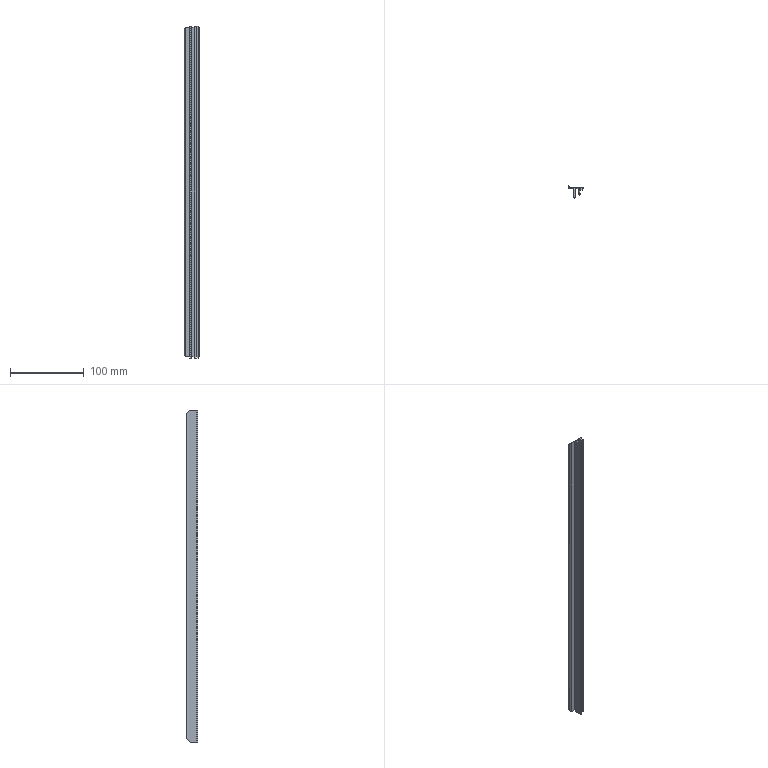Part | NX | features BREP 1 | 1 solid | 43 faces | box 21.266 x 16.173 x 450 mm | volume 30519 mm3 | plane 28 | cylinder 15 | commonest cylinder face diameters 0.585 x7 0.4 x2 1.951 x2 1.561 x1 8.16 x1 10.664 x1
STEP:
#1=CARTESIAN_POINT('',(0.,2.699,219.801));
#2=VERTEX_POINT('',#1);
#3=CARTESIAN_POINT('',(2.095,-0.55,223.05));
#4=VERTEX_POINT('',#3);
#5=CARTESIAN_POINT('',(0.,2.699,219.801));
#6=CARTESIAN_POINT('',(0.2706,1.376,221.124));
#7=CARTESIAN_POINT('',(1.002,0.242,222.258));
#8=CARTESIAN_POINT('',(2.095,-0.55,223.05));
#9=(BOUNDED_CURVE()B_SPLINE_CURVE(3,(#5,#6,#7,#8),.UNSPECIFIED.,.F.,.F.)B_SPLINE_CURVE_WITH_KNOTS((4,4),(1.773,2.515),.UNSPECIFIED.)CURVE()GEOMETRIC_REPRESENTATION_ITEM()RATIONAL_B_SPLINE_CURVE((1.,0.9547,0.9547,1.))REPRESENTATION_ITEM(''));
#10=EDGE_CURVE('',#2,#4,#9,.T.);
#11=ORIENTED_EDGE('',*,*,#10,.F.);
#12=CARTESIAN_POINT('',(0.,2.699,-219.801));
#13=VERTEX_POINT('',#12);
#14=CARTESIAN_POINT('',(0.,2.699,225.));
#15=DIRECTION('',(0.,0.,-1.));
#16=VECTOR('',#15,1000.);
#17=LINE('',#14,#16);
#18=EDGE_CURVE('',#2,#13,#17,.T.);
#19=ORIENTED_EDGE('',*,*,#18,.T.);
#20=CARTESIAN_POINT('',(2.095,-0.55,-223.05));
#21=VERTEX_POINT('',#20);
#22=CARTESIAN_POINT('',(2.095,-0.55,-223.05));
#23=CARTESIAN_POINT('',(1.002,0.242,-222.258));
#24=CARTESIAN_POINT('',(0.2706,1.376,-221.124));
#25=CARTESIAN_POINT('',(0.,2.699,-219.801));
#26=(BOUNDED_CURVE()B_SPLINE_CURVE(3,(#22,#23,#24,#25),.UNSPECIFIED.,.F.,.F.)B_SPLINE_CURVE_WITH_KNOTS((4,4),(0.6271,1.369),.UNSPECIFIED.)CURVE()GEOMETRIC_REPRESENTATION_ITEM()RATIONAL_B_SPLINE_CURVE((1.,0.9547,0.9547,1.))REPRESENTATION_ITEM(''));
#27=EDGE_CURVE('',#21,#13,#26,.T.);
#28=ORIENTED_EDGE('',*,*,#27,.F.);
#29=CARTESIAN_POINT('',(2.095,-0.55,225.));
#30=DIRECTION('',(0.,0.,-1.));
#31=VECTOR('',#30,1000.);
#32=LINE('',#29,#31);
#33=EDGE_CURVE('',#4,#21,#32,.T.);
#34=ORIENTED_EDGE('',*,*,#33,.F.);
#35=EDGE_LOOP('',(#11,#19,#28,#34));
#36=FACE_BOUND('',#35,.T.);
#37=CARTESIAN_POINT('',(5.224,3.768,225.));
#38=DIRECTION('',(0.,0.,-1.));
#39=DIRECTION('',(-1.,0.,0.));
#40=AXIS2_PLACEMENT_3D('',#37,#38,#39);
#41=CYLINDRICAL_SURFACE('',#40,5.332);
#42=ADVANCED_FACE('',(#36),#41,.T.);
#43=CARTESIAN_POINT('',(7.9,-0.55,223.05));
#44=VERTEX_POINT('',#43);
#45=CARTESIAN_POINT('',(2.095,-0.55,223.05));
#46=DIRECTION('',(1.,0.,0.));
#47=VECTOR('',#46,1000.);
#48=LINE('',#45,#47);
#49=EDGE_CURVE('',#4,#44,#48,.T.);
#50=ORIENTED_EDGE('',*,*,#49,.F.);
#51=ORIENTED_EDGE('',*,*,#33,.T.);
#52=CARTESIAN_POINT('',(7.9,-0.55,-223.05));
#53=VERTEX_POINT('',#52);
#54=CARTESIAN_POINT('',(2.095,-0.55,-223.05));
#55=DIRECTION('',(-1.,0.,0.));
#56=VECTOR('',#55,1000.);
#57=LINE('',#54,#56);
#58=EDGE_CURVE('',#53,#21,#57,.T.);
#59=ORIENTED_EDGE('',*,*,#58,.F.);
#60=CARTESIAN_POINT('',(7.9,-0.55,225.));
#61=DIRECTION('',(0.,0.,-1.));
#62=VECTOR('',#61,1000.);
#63=LINE('',#60,#62);
#64=EDGE_CURVE('',#44,#53,#63,.T.);
#65=ORIENTED_EDGE('',*,*,#64,.F.);
#66=EDGE_LOOP('',(#50,#51,#59,#65));
#67=FACE_BOUND('',#66,.T.);
#68=CARTESIAN_POINT('',(2.095,-0.55,225.));
#69=DIRECTION('',(0.,1.,0.));
#70=DIRECTION('',(1.,0.,0.));
#71=AXIS2_PLACEMENT_3D('',#68,#69,#70);
#72=PLANE('',#71);
#73=ADVANCED_FACE('',(#67),#72,.F.);
#74=CARTESIAN_POINT('',(7.9,-2.5,225.));
#75=VERTEX_POINT('',#74);
#76=CARTESIAN_POINT('',(7.9,-1.525,224.025));
#77=DIRECTION('',(0.,-0.7071,0.7071));
#78=VECTOR('',#77,1000.);
#79=LINE('',#76,#78);
#80=EDGE_CURVE('',#44,#75,#79,.T.);
#81=ORIENTED_EDGE('',*,*,#80,.F.);
#82=ORIENTED_EDGE('',*,*,#64,.T.);
#83=CARTESIAN_POINT('',(7.9,-2.5,-225.));
#84=VERTEX_POINT('',#83);
#85=CARTESIAN_POINT('',(7.9,223.475,0.975));
#86=DIRECTION('',(0.,0.7071,0.7071));
#87=VECTOR('',#86,1000.);
#88=LINE('',#85,#87);
#89=EDGE_CURVE('',#84,#53,#88,.T.);
#90=ORIENTED_EDGE('',*,*,#89,.F.);
#91=CARTESIAN_POINT('',(7.9,-11.847,-225.));
#92=VERTEX_POINT('',#91);
#93=CARTESIAN_POINT('',(7.9,-0.55,-225.));
#94=DIRECTION('',(0.,-1.,0.));
#95=VECTOR('',#94,1000.);
#96=LINE('',#93,#95);
#97=EDGE_CURVE('',#84,#92,#96,.T.);
#98=ORIENTED_EDGE('',*,*,#97,.T.);
#99=CARTESIAN_POINT('',(7.9,-11.847,225.));
#100=VERTEX_POINT('',#99);
#101=CARTESIAN_POINT('',(7.9,-11.847,225.));
#102=DIRECTION('',(0.,0.,-1.));
#103=VECTOR('',#102,1000.);
#104=LINE('',#101,#103);
#105=EDGE_CURVE('',#100,#92,#104,.T.);
#106=ORIENTED_EDGE('',*,*,#105,.F.);
#107=CARTESIAN_POINT('',(7.9,-0.55,225.));
#108=DIRECTION('',(0.,-1.,0.));
#109=VECTOR('',#108,1000.);
#110=LINE('',#107,#109);
#111=EDGE_CURVE('',#75,#100,#110,.T.);
#112=ORIENTED_EDGE('',*,*,#111,.F.);
#113=EDGE_LOOP('',(#81,#82,#90,#98,#106,#112));
#114=FACE_BOUND('',#113,.T.);
#115=CARTESIAN_POINT('',(7.9,-0.55,225.));
#116=DIRECTION('',(1.,0.,0.));
#117=DIRECTION('',(0.,1.,0.));
#118=AXIS2_PLACEMENT_3D('',#115,#116,#117);
#119=PLANE('',#118);
#120=ADVANCED_FACE('',(#114),#119,.F.);
#121=CARTESIAN_POINT('',(9.363,-2.5,225.));
#122=VERTEX_POINT('',#121);
#123=CARTESIAN_POINT('',(9.363,-1.526,224.026));
#124=VERTEX_POINT('',#123);
#125=CARTESIAN_POINT('',(9.363,-7.399,229.899));
#126=DIRECTION('',(0.,0.7071,-0.7071));
#127=VECTOR('',#126,1000.);
#128=LINE('',#125,#127);
#129=EDGE_CURVE('',#122,#124,#128,.T.);
#130=ORIENTED_EDGE('',*,*,#129,.F.);
#131=CARTESIAN_POINT('',(9.363,-12.298,225.));
#132=VERTEX_POINT('',#131);
#133=CARTESIAN_POINT('',(9.363,-12.298,225.));
#134=DIRECTION('',(0.,1.,0.));
#135=VECTOR('',#134,1000.);
#136=LINE('',#133,#135);
#137=EDGE_CURVE('',#132,#122,#136,.T.);
#138=ORIENTED_EDGE('',*,*,#137,.F.);
#139=CARTESIAN_POINT('',(9.363,-12.298,-225.));
#140=VERTEX_POINT('',#139);
#141=CARTESIAN_POINT('',(9.363,-12.298,225.));
#142=DIRECTION('',(0.,0.,-1.));
#143=VECTOR('',#142,1000.);
#144=LINE('',#141,#143);
#145=EDGE_CURVE('',#132,#140,#144,.T.);
#146=ORIENTED_EDGE('',*,*,#145,.T.);
#147=CARTESIAN_POINT('',(9.363,-2.5,-225.));
#148=VERTEX_POINT('',#147);
#149=CARTESIAN_POINT('',(9.363,-12.298,-225.));
#150=DIRECTION('',(0.,1.,0.));
#151=VECTOR('',#150,1000.);
#152=LINE('',#149,#151);
#153=EDGE_CURVE('',#140,#148,#152,.T.);
#154=ORIENTED_EDGE('',*,*,#153,.T.);
#155=CARTESIAN_POINT('',(9.363,-1.526,-224.026));
#156=VERTEX_POINT('',#155);
#157=CARTESIAN_POINT('',(9.363,217.601,-4.899));
#158=DIRECTION('',(0.,-0.7071,-0.7071));
#159=VECTOR('',#158,1000.);
#160=LINE('',#157,#159);
#161=EDGE_CURVE('',#156,#148,#160,.T.);
#162=ORIENTED_EDGE('',*,*,#161,.F.);
#163=CARTESIAN_POINT('',(9.363,-1.526,225.));
#164=DIRECTION('',(0.,0.,-1.));
#165=VECTOR('',#164,1000.);
#166=LINE('',#163,#165);
#167=EDGE_CURVE('',#124,#156,#166,.T.);
#168=ORIENTED_EDGE('',*,*,#167,.F.);
#169=EDGE_LOOP('',(#130,#138,#146,#154,#162,#168));
#170=FACE_BOUND('',#169,.T.);
#171=CARTESIAN_POINT('',(9.363,-12.298,225.));
#172=DIRECTION('',(-1.,0.,0.));
#173=DIRECTION('',(0.,0.,1.));
#174=AXIS2_PLACEMENT_3D('',#171,#172,#173);
#175=PLANE('',#174);
#176=ADVANCED_FACE('',(#170),#175,.F.);
#177=CARTESIAN_POINT('',(10.339,-0.55,223.05));
#178=VERTEX_POINT('',#177);
#179=CARTESIAN_POINT('',(9.363,-1.526,224.026));
#180=CARTESIAN_POINT('',(9.363,-0.9541,223.454));
#181=CARTESIAN_POINT('',(9.768,-0.55,223.05));
#182=CARTESIAN_POINT('',(10.339,-0.55,223.05));
#183=(BOUNDED_CURVE()B_SPLINE_CURVE(3,(#179,#180,#181,#182),.UNSPECIFIED.,.F.,.F.)B_SPLINE_CURVE_WITH_KNOTS((4,4),(4.712,6.283),.UNSPECIFIED.)CURVE()GEOMETRIC_REPRESENTATION_ITEM()RATIONAL_B_SPLINE_CURVE((1.,0.8047,0.8047,1.))REPRESENTATION_ITEM(''));
#184=EDGE_CURVE('',#124,#178,#183,.T.);
#185=ORIENTED_EDGE('',*,*,#184,.F.);
#186=ORIENTED_EDGE('',*,*,#167,.T.);
#187=CARTESIAN_POINT('',(10.339,-0.55,-223.05));
#188=VERTEX_POINT('',#187);
#189=CARTESIAN_POINT('',(10.339,-0.55,-223.05));
#190=CARTESIAN_POINT('',(9.768,-0.55,-223.05));
#191=CARTESIAN_POINT('',(9.363,-0.9541,-223.454));
#192=CARTESIAN_POINT('',(9.363,-1.526,-224.026));
#193=(BOUNDED_CURVE()B_SPLINE_CURVE(3,(#189,#190,#191,#192),.UNSPECIFIED.,.F.,.F.)B_SPLINE_CURVE_WITH_KNOTS((4,4),(3.142,4.712),.UNSPECIFIED.)CURVE()GEOMETRIC_REPRESENTATION_ITEM()RATIONAL_B_SPLINE_CURVE((1.,0.8047,0.8047,1.))REPRESENTATION_ITEM(''));
#194=EDGE_CURVE('',#188,#156,#193,.T.);
#195=ORIENTED_EDGE('',*,*,#194,.F.);
#196=CARTESIAN_POINT('',(10.339,-0.55,225.));
#197=DIRECTION('',(0.,0.,-1.));
#198=VECTOR('',#197,1000.);
#199=LINE('',#196,#198);
#200=EDGE_CURVE('',#178,#188,#199,.T.);
#201=ORIENTED_EDGE('',*,*,#200,.F.);
#202=EDGE_LOOP('',(#185,#186,#195,#201));
#203=FACE_BOUND('',#202,.T.);
#204=CARTESIAN_POINT('',(10.339,-1.526,225.));
#205=DIRECTION('',(0.,0.,-1.));
#206=DIRECTION('',(-1.,0.,0.));
#207=AXIS2_PLACEMENT_3D('',#204,#205,#206);
#208=CYLINDRICAL_SURFACE('',#207,0.9756);
#209=ADVANCED_FACE('',(#203),#208,.F.);
#210=CARTESIAN_POINT('',(13.461,-0.55,223.05));
#211=VERTEX_POINT('',#210);
#212=CARTESIAN_POINT('',(10.339,-0.55,223.05));
#213=DIRECTION('',(1.,0.,0.));
#214=VECTOR('',#213,1000.);
#215=LINE('',#212,#214);
#216=EDGE_CURVE('',#178,#211,#215,.T.);
#217=ORIENTED_EDGE('',*,*,#216,.F.);
#218=ORIENTED_EDGE('',*,*,#200,.T.);
#219=CARTESIAN_POINT('',(13.461,-0.55,-223.05));
#220=VERTEX_POINT('',#219);
#221=CARTESIAN_POINT('',(10.339,-0.55,-223.05));
#222=DIRECTION('',(-1.,0.,0.));
#223=VECTOR('',#222,1000.);
#224=LINE('',#221,#223);
#225=EDGE_CURVE('',#220,#188,#224,.T.);
#226=ORIENTED_EDGE('',*,*,#225,.F.);
#227=CARTESIAN_POINT('',(13.461,-0.55,225.));
#228=DIRECTION('',(0.,0.,-1.));
#229=VECTOR('',#228,1000.);
#230=LINE('',#227,#229);
#231=EDGE_CURVE('',#211,#220,#230,.T.);
#232=ORIENTED_EDGE('',*,*,#231,.F.);
#233=EDGE_LOOP('',(#217,#218,#226,#232));
#234=FACE_BOUND('',#233,.T.);
#235=CARTESIAN_POINT('',(10.339,-0.55,225.));
#236=DIRECTION('',(0.,1.,0.));
#237=DIRECTION('',(1.,0.,0.));
#238=AXIS2_PLACEMENT_3D('',#235,#236,#237);
#239=PLANE('',#238);
#240=ADVANCED_FACE('',(#234),#239,.F.);
#241=CARTESIAN_POINT('',(14.437,-1.526,224.026));
#242=VERTEX_POINT('',#241);
#243=CARTESIAN_POINT('',(13.461,-0.55,223.05));
#244=CARTESIAN_POINT('',(14.032,-0.55,223.05));
#245=CARTESIAN_POINT('',(14.437,-0.9541,223.454));
#246=CARTESIAN_POINT('',(14.437,-1.526,224.026));
#247=(BOUNDED_CURVE()B_SPLINE_CURVE(3,(#243,#244,#245,#246),.UNSPECIFIED.,.F.,.F.)B_SPLINE_CURVE_WITH_KNOTS((4,4),(0.,1.571),.UNSPECIFIED.)CURVE()GEOMETRIC_REPRESENTATION_ITEM()RATIONAL_B_SPLINE_CURVE((1.,0.8047,0.8047,1.))REPRESENTATION_ITEM(''));
#248=EDGE_CURVE('',#211,#242,#247,.T.);
#249=ORIENTED_EDGE('',*,*,#248,.F.);
#250=ORIENTED_EDGE('',*,*,#231,.T.);
#251=CARTESIAN_POINT('',(14.437,-1.526,-224.026));
#252=VERTEX_POINT('',#251);
#253=CARTESIAN_POINT('',(14.437,-1.526,-224.026));
#254=CARTESIAN_POINT('',(14.437,-0.9541,-223.454));
#255=CARTESIAN_POINT('',(14.032,-0.55,-223.05));
#256=CARTESIAN_POINT('',(13.461,-0.55,-223.05));
#257=(BOUNDED_CURVE()B_SPLINE_CURVE(3,(#253,#254,#255,#256),.UNSPECIFIED.,.F.,.F.)B_SPLINE_CURVE_WITH_KNOTS((4,4),(1.571,3.142),.UNSPECIFIED.)CURVE()GEOMETRIC_REPRESENTATION_ITEM()RATIONAL_B_SPLINE_CURVE((1.,0.8047,0.8047,1.))REPRESENTATION_ITEM(''));
#258=EDGE_CURVE('',#252,#220,#257,.T.);
#259=ORIENTED_EDGE('',*,*,#258,.F.);
#260=CARTESIAN_POINT('',(14.437,-1.526,225.));
#261=DIRECTION('',(0.,0.,-1.));
#262=VECTOR('',#261,1000.);
#263=LINE('',#260,#262);
#264=EDGE_CURVE('',#242,#252,#263,.T.);
#265=ORIENTED_EDGE('',*,*,#264,.F.);
#266=EDGE_LOOP('',(#249,#250,#259,#265));
#267=FACE_BOUND('',#266,.T.);
#268=CARTESIAN_POINT('',(13.461,-1.526,225.));
#269=DIRECTION('',(0.,0.,-1.));
#270=DIRECTION('',(-1.,0.,0.));
#271=AXIS2_PLACEMENT_3D('',#268,#269,#270);
#272=CYLINDRICAL_SURFACE('',#271,0.9756);
#273=ADVANCED_FACE('',(#267),#272,.F.);
#274=CARTESIAN_POINT('',(14.437,-2.5,225.));
#275=VERTEX_POINT('',#274);
#276=CARTESIAN_POINT('',(14.437,-2.013,224.513));
#277=DIRECTION('',(0.,-0.7071,0.7071));
#278=VECTOR('',#277,1000.);
#279=LINE('',#276,#278);
#280=EDGE_CURVE('',#242,#275,#279,.T.);
#281=ORIENTED_EDGE('',*,*,#280,.F.);
#282=ORIENTED_EDGE('',*,*,#264,.T.);
#283=CARTESIAN_POINT('',(14.437,-2.5,-225.));
#284=VERTEX_POINT('',#283);
#285=CARTESIAN_POINT('',(14.437,222.987,0.4872));
#286=DIRECTION('',(0.,0.7071,0.7071));
#287=VECTOR('',#286,1000.);
#288=LINE('',#285,#287);
#289=EDGE_CURVE('',#284,#252,#288,.T.);
#290=ORIENTED_EDGE('',*,*,#289,.F.);
#291=CARTESIAN_POINT('',(14.437,-8.128,-225.));
#292=VERTEX_POINT('',#291);
#293=CARTESIAN_POINT('',(14.437,-1.526,-225.));
#294=DIRECTION('',(0.,-1.,0.));
#295=VECTOR('',#294,1000.);
#296=LINE('',#293,#295);
#297=EDGE_CURVE('',#284,#292,#296,.T.);
#298=ORIENTED_EDGE('',*,*,#297,.T.);
#299=CARTESIAN_POINT('',(14.437,-8.128,225.));
#300=VERTEX_POINT('',#299);
#301=CARTESIAN_POINT('',(14.437,-8.128,225.));
#302=DIRECTION('',(0.,0.,-1.));
#303=VECTOR('',#302,1000.);
#304=LINE('',#301,#303);
#305=EDGE_CURVE('',#300,#292,#304,.T.);
#306=ORIENTED_EDGE('',*,*,#305,.F.);
#307=CARTESIAN_POINT('',(14.437,-1.526,225.));
#308=DIRECTION('',(0.,-1.,0.));
#309=VECTOR('',#308,1000.);
#310=LINE('',#307,#309);
#311=EDGE_CURVE('',#275,#300,#310,.T.);
#312=ORIENTED_EDGE('',*,*,#311,.F.);
#313=EDGE_LOOP('',(#281,#282,#290,#298,#306,#312));
#314=FACE_BOUND('',#313,.T.);
#315=CARTESIAN_POINT('',(14.437,-1.526,225.));
#316=DIRECTION('',(1.,0.,0.));
#317=DIRECTION('',(0.,1.,0.));
#318=AXIS2_PLACEMENT_3D('',#315,#316,#317);
#319=PLANE('',#318);
#320=ADVANCED_FACE('',(#314),#319,.F.);
#321=CARTESIAN_POINT('',(15.9,-2.5,225.));
#322=VERTEX_POINT('',#321);
#323=CARTESIAN_POINT('',(15.9,-0.55,223.05));
#324=VERTEX_POINT('',#323);
#325=CARTESIAN_POINT('',(15.9,-4.93,227.43));
#326=DIRECTION('',(0.,0.7071,-0.7071));
#327=VECTOR('',#326,1000.);
#328=LINE('',#325,#327);
#329=EDGE_CURVE('',#322,#324,#328,.T.);
#330=ORIENTED_EDGE('',*,*,#329,.F.);
#331=CARTESIAN_POINT('',(15.9,-7.36,225.));
#332=VERTEX_POINT('',#331);
#333=CARTESIAN_POINT('',(15.9,-7.36,225.));
#334=DIRECTION('',(0.,1.,0.));
#335=VECTOR('',#334,1000.);
#336=LINE('',#333,#335);
#337=EDGE_CURVE('',#332,#322,#336,.T.);
#338=ORIENTED_EDGE('',*,*,#337,.F.);
#339=CARTESIAN_POINT('',(15.9,-7.36,-225.));
#340=VERTEX_POINT('',#339);
#341=CARTESIAN_POINT('',(15.9,-7.36,225.));
#342=DIRECTION('',(0.,0.,-1.));
#343=VECTOR('',#342,1000.);
#344=LINE('',#341,#343);
#345=EDGE_CURVE('',#332,#340,#344,.T.);
#346=ORIENTED_EDGE('',*,*,#345,.T.);
#347=CARTESIAN_POINT('',(15.9,-2.5,-225.));
#348=VERTEX_POINT('',#347);
#349=CARTESIAN_POINT('',(15.9,-7.36,-225.));
#350=DIRECTION('',(0.,1.,0.));
#351=VECTOR('',#350,1000.);
#352=LINE('',#349,#351);
#353=EDGE_CURVE('',#340,#348,#352,.T.);
#354=ORIENTED_EDGE('',*,*,#353,.T.);
#355=CARTESIAN_POINT('',(15.9,-0.55,-223.05));
#356=VERTEX_POINT('',#355);
#357=CARTESIAN_POINT('',(15.9,220.07,-2.43));
#358=DIRECTION('',(0.,-0.7071,-0.7071));
#359=VECTOR('',#358,1000.);
#360=LINE('',#357,#359);
#361=EDGE_CURVE('',#356,#348,#360,.T.);
#362=ORIENTED_EDGE('',*,*,#361,.F.);
#363=CARTESIAN_POINT('',(15.9,-0.55,225.));
#364=DIRECTION('',(0.,0.,-1.));
#365=VECTOR('',#364,1000.);
#366=LINE('',#363,#365);
#367=EDGE_CURVE('',#324,#356,#366,.T.);
#368=ORIENTED_EDGE('',*,*,#367,.F.);
#369=EDGE_LOOP('',(#330,#338,#346,#354,#362,#368));
#370=FACE_BOUND('',#369,.T.);
#371=CARTESIAN_POINT('',(15.9,-7.36,225.));
#372=DIRECTION('',(-1.,0.,0.));
#373=DIRECTION('',(0.,0.,1.));
#374=AXIS2_PLACEMENT_3D('',#371,#372,#373);
#375=PLANE('',#374);
#376=ADVANCED_FACE('',(#370),#375,.F.);
#377=CARTESIAN_POINT('',(17.363,-0.55,223.05));
#378=VERTEX_POINT('',#377);
#379=CARTESIAN_POINT('',(15.9,-0.55,223.05));
#380=DIRECTION('',(1.,0.,0.));
#381=VECTOR('',#380,1000.);
#382=LINE('',#379,#381);
#383=EDGE_CURVE('',#324,#378,#382,.T.);
#384=ORIENTED_EDGE('',*,*,#383,.F.);
#385=ORIENTED_EDGE('',*,*,#367,.T.);
#386=CARTESIAN_POINT('',(17.363,-0.55,-223.05));
#387=VERTEX_POINT('',#386);
#388=CARTESIAN_POINT('',(15.9,-0.55,-223.05));
#389=DIRECTION('',(-1.,0.,0.));
#390=VECTOR('',#389,1000.);
#391=LINE('',#388,#390);
#392=EDGE_CURVE('',#387,#356,#391,.T.);
#393=ORIENTED_EDGE('',*,*,#392,.F.);
#394=CARTESIAN_POINT('',(17.363,-0.55,225.));
#395=DIRECTION('',(0.,0.,-1.));
#396=VECTOR('',#395,1000.);
#397=LINE('',#394,#396);
#398=EDGE_CURVE('',#378,#387,#397,.T.);
#399=ORIENTED_EDGE('',*,*,#398,.F.);
#400=EDGE_LOOP('',(#384,#385,#393,#399));
#401=FACE_BOUND('',#400,.T.);
#402=CARTESIAN_POINT('',(15.9,-0.55,225.));
#403=DIRECTION('',(0.,1.,0.));
#404=DIRECTION('',(1.,0.,0.));
#405=AXIS2_PLACEMENT_3D('',#402,#403,#404);
#406=PLANE('',#405);
#407=ADVANCED_FACE('',(#401),#406,.F.);
#408=CARTESIAN_POINT('',(17.363,-2.5,225.));
#409=VERTEX_POINT('',#408);
#410=CARTESIAN_POINT('',(17.363,-1.525,224.025));
#411=DIRECTION('',(0.,-0.7071,0.7071));
#412=VECTOR('',#411,1000.);
#413=LINE('',#410,#412);
#414=EDGE_CURVE('',#378,#409,#413,.T.);
#415=ORIENTED_EDGE('',*,*,#414,.F.);
#416=ORIENTED_EDGE('',*,*,#398,.T.);
#417=CARTESIAN_POINT('',(17.363,-2.5,-225.));
#418=VERTEX_POINT('',#417);
#419=CARTESIAN_POINT('',(17.363,223.475,0.975));
#420=DIRECTION('',(0.,0.7071,0.7071));
#421=VECTOR('',#420,1000.);
#422=LINE('',#419,#421);
#423=EDGE_CURVE('',#418,#387,#422,.T.);
#424=ORIENTED_EDGE('',*,*,#423,.F.);
#425=CARTESIAN_POINT('',(17.363,-2.501,-225.));
#426=VERTEX_POINT('',#425);
#427=CARTESIAN_POINT('',(17.363,-0.55,-225.));
#428=DIRECTION('',(0.,-1.,0.));
#429=VECTOR('',#428,1000.);
#430=LINE('',#427,#429);
#431=EDGE_CURVE('',#418,#426,#430,.T.);
#432=ORIENTED_EDGE('',*,*,#431,.T.);
#433=CARTESIAN_POINT('',(17.363,-2.501,225.));
#434=VERTEX_POINT('',#433);
#435=CARTESIAN_POINT('',(17.363,-2.501,225.));
#436=DIRECTION('',(0.,0.,-1.));
#437=VECTOR('',#436,1000.);
#438=LINE('',#435,#437);
#439=EDGE_CURVE('',#434,#426,#438,.T.);
#440=ORIENTED_EDGE('',*,*,#439,.F.);
#441=CARTESIAN_POINT('',(17.363,-0.55,225.));
#442=DIRECTION('',(0.,-1.,0.));
#443=VECTOR('',#442,1000.);
#444=LINE('',#441,#443);
#445=EDGE_CURVE('',#409,#434,#444,.T.);
#446=ORIENTED_EDGE('',*,*,#445,.F.);
#447=EDGE_LOOP('',(#415,#416,#424,#432,#440,#446));
#448=FACE_BOUND('',#447,.T.);
#449=CARTESIAN_POINT('',(17.363,-0.55,225.));
#450=DIRECTION('',(1.,0.,0.));
#451=DIRECTION('',(0.,1.,0.));
#452=AXIS2_PLACEMENT_3D('',#449,#450,#451);
#453=PLANE('',#452);
#454=ADVANCED_FACE('',(#448),#453,.F.);
#455=CARTESIAN_POINT('',(19.049,-2.5,225.));
#456=VERTEX_POINT('',#455);
#457=CARTESIAN_POINT('',(19.315,-2.209,224.709));
#458=VERTEX_POINT('',#457);
#459=CARTESIAN_POINT('',(19.049,-2.5,225.));
#460=CARTESIAN_POINT('',(19.207,-2.485,224.985));
#461=CARTESIAN_POINT('',(19.315,-2.368,224.868));
#462=CARTESIAN_POINT('',(19.315,-2.209,224.709));
#463=(BOUNDED_CURVE()B_SPLINE_CURVE(3,(#459,#460,#461,#462),.UNSPECIFIED.,.F.,.F.)B_SPLINE_CURVE_WITH_KNOTS((4,4),(3.233,4.712),.UNSPECIFIED.)CURVE()GEOMETRIC_REPRESENTATION_ITEM()RATIONAL_B_SPLINE_CURVE((1.,0.8258,0.8258,1.))REPRESENTATION_ITEM(''));
#464=EDGE_CURVE('',#456,#458,#463,.T.);
#465=ORIENTED_EDGE('',*,*,#464,.F.);
#466=CARTESIAN_POINT('',(19.022,-2.501,225.));
#467=VERTEX_POINT('',#466);
#468=CARTESIAN_POINT('',(19.022,-2.209,225.));
#469=DIRECTION('',(0.,0.,1.));
#470=DIRECTION('',(1.,0.,0.));
#471=AXIS2_PLACEMENT_3D('',#468,#469,#470);
#472=CIRCLE('',#471,0.2927);
#473=EDGE_CURVE('',#467,#456,#472,.T.);
#474=ORIENTED_EDGE('',*,*,#473,.F.);
#475=CARTESIAN_POINT('',(19.022,-2.501,-225.));
#476=VERTEX_POINT('',#475);
#477=CARTESIAN_POINT('',(19.022,-2.501,225.));
#478=DIRECTION('',(0.,0.,-1.));
#479=VECTOR('',#478,1000.);
#480=LINE('',#477,#479);
#481=EDGE_CURVE('',#467,#476,#480,.T.);
#482=ORIENTED_EDGE('',*,*,#481,.T.);
#483=CARTESIAN_POINT('',(19.049,-2.5,-225.));
#484=VERTEX_POINT('',#483);
#485=CARTESIAN_POINT('',(19.022,-2.209,-225.));
#486=DIRECTION('',(0.,0.,1.));
#487=DIRECTION('',(1.,0.,0.));
#488=AXIS2_PLACEMENT_3D('',#485,#486,#487);
#489=CIRCLE('',#488,0.2927);
#490=EDGE_CURVE('',#476,#484,#489,.T.);
#491=ORIENTED_EDGE('',*,*,#490,.T.);
#492=CARTESIAN_POINT('',(19.315,-2.209,-224.709));
#493=VERTEX_POINT('',#492);
#494=CARTESIAN_POINT('',(19.315,-2.209,-224.709));
#495=CARTESIAN_POINT('',(19.315,-2.368,-224.868));
#496=CARTESIAN_POINT('',(19.207,-2.485,-224.985));
#497=CARTESIAN_POINT('',(19.049,-2.5,-225.));
#498=(BOUNDED_CURVE()B_SPLINE_CURVE(3,(#494,#495,#496,#497),.UNSPECIFIED.,.F.,.F.)B_SPLINE_CURVE_WITH_KNOTS((4,4),(4.712,6.192),.UNSPECIFIED.)CURVE()GEOMETRIC_REPRESENTATION_ITEM()RATIONAL_B_SPLINE_CURVE((1.,0.8258,0.8258,1.))REPRESENTATION_ITEM(''));
#499=EDGE_CURVE('',#493,#484,#498,.T.);
#500=ORIENTED_EDGE('',*,*,#499,.F.);
#501=CARTESIAN_POINT('',(19.315,-2.209,225.));
#502=DIRECTION('',(0.,0.,-1.));
#503=VECTOR('',#502,1000.);
#504=LINE('',#501,#503);
#505=EDGE_CURVE('',#458,#493,#504,.T.);
#506=ORIENTED_EDGE('',*,*,#505,.F.);
#507=EDGE_LOOP('',(#465,#474,#482,#491,#500,#506));
#508=FACE_BOUND('',#507,.T.);
#509=CARTESIAN_POINT('',(19.022,-2.209,225.));
#510=DIRECTION('',(0.,0.,-1.));
#511=DIRECTION('',(-1.,0.,0.));
#512=AXIS2_PLACEMENT_3D('',#509,#510,#511);
#513=CYLINDRICAL_SURFACE('',#512,0.2927);
#514=ADVANCED_FACE('',(#508),#513,.T.);
#515=CARTESIAN_POINT('',(19.315,-0.8427,223.343));
#516=VERTEX_POINT('',#515);
#517=CARTESIAN_POINT('',(19.315,-2.354,224.854));
#518=DIRECTION('',(0.,0.7071,-0.7071));
#519=VECTOR('',#518,1000.);
#520=LINE('',#517,#519);
#521=EDGE_CURVE('',#458,#516,#520,.T.);
#522=ORIENTED_EDGE('',*,*,#521,.F.);
#523=ORIENTED_EDGE('',*,*,#505,.T.);
#524=CARTESIAN_POINT('',(19.315,-0.8427,-223.343));
#525=VERTEX_POINT('',#524);
#526=CARTESIAN_POINT('',(19.315,222.646,0.1457));
#527=DIRECTION('',(0.,-0.7071,-0.7071));
#528=VECTOR('',#527,1000.);
#529=LINE('',#526,#528);
#530=EDGE_CURVE('',#525,#493,#529,.T.);
#531=ORIENTED_EDGE('',*,*,#530,.F.);
#532=CARTESIAN_POINT('',(19.315,-0.8427,225.));
#533=DIRECTION('',(0.,0.,-1.));
#534=VECTOR('',#533,1000.);
#535=LINE('',#532,#534);
#536=EDGE_CURVE('',#516,#525,#535,.T.);
#537=ORIENTED_EDGE('',*,*,#536,.F.);
#538=EDGE_LOOP('',(#522,#523,#531,#537));
#539=FACE_BOUND('',#538,.T.);
#540=CARTESIAN_POINT('',(19.315,-2.209,225.));
#541=DIRECTION('',(-1.,0.,0.));
#542=DIRECTION('',(0.,0.,1.));
#543=AXIS2_PLACEMENT_3D('',#540,#541,#542);
#544=PLANE('',#543);
#545=ADVANCED_FACE('',(#539),#544,.F.);
#546=CARTESIAN_POINT('',(19.607,-0.55,223.05));
#547=VERTEX_POINT('',#546);
#548=CARTESIAN_POINT('',(19.315,-0.8427,223.343));
#549=CARTESIAN_POINT('',(19.315,-0.6712,223.171));
#550=CARTESIAN_POINT('',(19.436,-0.55,223.05));
#551=CARTESIAN_POINT('',(19.607,-0.55,223.05));
#552=(BOUNDED_CURVE()B_SPLINE_CURVE(3,(#548,#549,#550,#551),.UNSPECIFIED.,.F.,.F.)B_SPLINE_CURVE_WITH_KNOTS((4,4),(4.712,6.283),.UNSPECIFIED.)CURVE()GEOMETRIC_REPRESENTATION_ITEM()RATIONAL_B_SPLINE_CURVE((1.,0.8047,0.8047,1.))REPRESENTATION_ITEM(''));
#553=EDGE_CURVE('',#516,#547,#552,.T.);
#554=ORIENTED_EDGE('',*,*,#553,.F.);
#555=ORIENTED_EDGE('',*,*,#536,.T.);
#556=CARTESIAN_POINT('',(19.607,-0.55,-223.05));
#557=VERTEX_POINT('',#556);
#558=CARTESIAN_POINT('',(19.607,-0.55,-223.05));
#559=CARTESIAN_POINT('',(19.436,-0.55,-223.05));
#560=CARTESIAN_POINT('',(19.315,-0.6712,-223.171));
#561=CARTESIAN_POINT('',(19.315,-0.8427,-223.343));
#562=(BOUNDED_CURVE()B_SPLINE_CURVE(3,(#558,#559,#560,#561),.UNSPECIFIED.,.F.,.F.)B_SPLINE_CURVE_WITH_KNOTS((4,4),(3.142,4.712),.UNSPECIFIED.)CURVE()GEOMETRIC_REPRESENTATION_ITEM()RATIONAL_B_SPLINE_CURVE((1.,0.8047,0.8047,1.))REPRESENTATION_ITEM(''));
#563=EDGE_CURVE('',#557,#525,#562,.T.);
#564=ORIENTED_EDGE('',*,*,#563,.F.);
#565=CARTESIAN_POINT('',(19.607,-0.55,225.));
#566=DIRECTION('',(0.,0.,-1.));
#567=VECTOR('',#566,1000.);
#568=LINE('',#565,#567);
#569=EDGE_CURVE('',#547,#557,#568,.T.);
#570=ORIENTED_EDGE('',*,*,#569,.F.);
#571=EDGE_LOOP('',(#554,#555,#564,#570));
#572=FACE_BOUND('',#571,.T.);
#573=CARTESIAN_POINT('',(19.607,-0.8427,225.));
#574=DIRECTION('',(0.,0.,-1.));
#575=DIRECTION('',(-1.,0.,0.));
#576=AXIS2_PLACEMENT_3D('',#573,#574,#575);
#577=CYLINDRICAL_SURFACE('',#576,0.2927);
#578=ADVANCED_FACE('',(#572),#577,.F.);
#579=CARTESIAN_POINT('',(20.973,-0.55,223.05));
#580=VERTEX_POINT('',#579);
#581=CARTESIAN_POINT('',(19.607,-0.55,223.05));
#582=DIRECTION('',(1.,0.,0.));
#583=VECTOR('',#582,1000.);
#584=LINE('',#581,#583);
#585=EDGE_CURVE('',#547,#580,#584,.T.);
#586=ORIENTED_EDGE('',*,*,#585,.F.);
#587=ORIENTED_EDGE('',*,*,#569,.T.);
#588=CARTESIAN_POINT('',(20.973,-0.55,-223.05));
#589=VERTEX_POINT('',#588);
#590=CARTESIAN_POINT('',(19.607,-0.55,-223.05));
#591=DIRECTION('',(-1.,0.,0.));
#592=VECTOR('',#591,1000.);
#593=LINE('',#590,#592);
#594=EDGE_CURVE('',#589,#557,#593,.T.);
#595=ORIENTED_EDGE('',*,*,#594,.F.);
#596=CARTESIAN_POINT('',(20.973,-0.55,225.));
#597=DIRECTION('',(0.,0.,-1.));
#598=VECTOR('',#597,1000.);
#599=LINE('',#596,#598);
#600=EDGE_CURVE('',#580,#589,#599,.T.);
#601=ORIENTED_EDGE('',*,*,#600,.F.);
#602=EDGE_LOOP('',(#586,#587,#595,#601));
#603=FACE_BOUND('',#602,.T.);
#604=CARTESIAN_POINT('',(19.607,-0.55,225.));
#605=DIRECTION('',(0.,1.,0.));
#606=DIRECTION('',(1.,0.,0.));
#607=AXIS2_PLACEMENT_3D('',#604,#605,#606);
#608=PLANE('',#607);
#609=ADVANCED_FACE('',(#603),#608,.F.);
#610=CARTESIAN_POINT('',(21.266,-0.2573,222.757));
#611=VERTEX_POINT('',#610);
#612=CARTESIAN_POINT('',(20.973,-0.55,223.05));
#613=CARTESIAN_POINT('',(21.145,-0.55,223.05));
#614=CARTESIAN_POINT('',(21.266,-0.4288,222.929));
#615=CARTESIAN_POINT('',(21.266,-0.2573,222.757));
#616=(BOUNDED_CURVE()B_SPLINE_CURVE(3,(#612,#613,#614,#615),.UNSPECIFIED.,.F.,.F.)B_SPLINE_CURVE_WITH_KNOTS((4,4),(3.142,4.712),.UNSPECIFIED.)CURVE()GEOMETRIC_REPRESENTATION_ITEM()RATIONAL_B_SPLINE_CURVE((1.,0.8047,0.8047,1.))REPRESENTATION_ITEM(''));
#617=EDGE_CURVE('',#580,#611,#616,.T.);
#618=ORIENTED_EDGE('',*,*,#617,.F.);
#619=ORIENTED_EDGE('',*,*,#600,.T.);
#620=CARTESIAN_POINT('',(21.266,-0.2573,-222.757));
#621=VERTEX_POINT('',#620);
#622=CARTESIAN_POINT('',(21.266,-0.2573,-222.757));
#623=CARTESIAN_POINT('',(21.266,-0.4288,-222.929));
#624=CARTESIAN_POINT('',(21.145,-0.55,-223.05));
#625=CARTESIAN_POINT('',(20.973,-0.55,-223.05));
#626=(BOUNDED_CURVE()B_SPLINE_CURVE(3,(#622,#623,#624,#625),.UNSPECIFIED.,.F.,.F.)B_SPLINE_CURVE_WITH_KNOTS((4,4),(4.712,6.283),.UNSPECIFIED.)CURVE()GEOMETRIC_REPRESENTATION_ITEM()RATIONAL_B_SPLINE_CURVE((1.,0.8047,0.8047,1.))REPRESENTATION_ITEM(''));
#627=EDGE_CURVE('',#621,#589,#626,.T.);
#628=ORIENTED_EDGE('',*,*,#627,.F.);
#629=CARTESIAN_POINT('',(21.266,-0.2573,225.));
#630=DIRECTION('',(0.,0.,-1.));
#631=VECTOR('',#630,1000.);
#632=LINE('',#629,#631);
#633=EDGE_CURVE('',#611,#621,#632,.T.);
#634=ORIENTED_EDGE('',*,*,#633,.F.);
#635=EDGE_LOOP('',(#618,#619,#628,#634));
#636=FACE_BOUND('',#635,.T.);
#637=CARTESIAN_POINT('',(20.973,-0.2573,225.));
#638=DIRECTION('',(0.,0.,-1.));
#639=DIRECTION('',(-1.,0.,0.));
#640=AXIS2_PLACEMENT_3D('',#637,#638,#639);
#641=CYLINDRICAL_SURFACE('',#640,0.2927);
#642=ADVANCED_FACE('',(#636),#641,.T.);
#643=CARTESIAN_POINT('',(21.266,0.8034,221.697));
#644=VERTEX_POINT('',#643);
#645=CARTESIAN_POINT('',(21.266,-2.5,225.));
#646=DIRECTION('',(0.,0.7071,-0.7071));
#647=VECTOR('',#646,1000.);
#648=LINE('',#645,#647);
#649=EDGE_CURVE('',#611,#644,#648,.T.);
#650=ORIENTED_EDGE('',*,*,#649,.F.);
#651=ORIENTED_EDGE('',*,*,#633,.T.);
#652=CARTESIAN_POINT('',(21.266,0.8034,-221.697));
#653=VERTEX_POINT('',#652);
#654=CARTESIAN_POINT('',(21.266,-2.5,-225.));
#655=DIRECTION('',(0.,-0.7071,-0.7071));
#656=VECTOR('',#655,1000.);
#657=LINE('',#654,#656);
#658=EDGE_CURVE('',#653,#621,#657,.T.);
#659=ORIENTED_EDGE('',*,*,#658,.F.);
#660=CARTESIAN_POINT('',(21.266,0.8034,225.));
#661=DIRECTION('',(0.,0.,-1.));
#662=VECTOR('',#661,1000.);
#663=LINE('',#660,#662);
#664=EDGE_CURVE('',#644,#653,#663,.T.);
#665=ORIENTED_EDGE('',*,*,#664,.F.);
#666=EDGE_LOOP('',(#650,#651,#659,#665));
#667=FACE_BOUND('',#666,.T.);
#668=CARTESIAN_POINT('',(21.266,-0.2573,225.));
#669=DIRECTION('',(-1.,0.,0.));
#670=DIRECTION('',(0.,0.,1.));
#671=AXIS2_PLACEMENT_3D('',#668,#669,#670);
#672=PLANE('',#671);
#673=ADVANCED_FACE('',(#667),#672,.F.);
#674=CARTESIAN_POINT('',(21.066,1.003,221.497));
#675=VERTEX_POINT('',#674);
#676=CARTESIAN_POINT('',(21.266,0.8034,221.697));
#677=CARTESIAN_POINT('',(21.266,0.9206,221.579));
#678=CARTESIAN_POINT('',(21.183,1.003,221.497));
#679=CARTESIAN_POINT('',(21.066,1.003,221.497));
#680=(BOUNDED_CURVE()B_SPLINE_CURVE(3,(#676,#677,#678,#679),.UNSPECIFIED.,.F.,.F.)B_SPLINE_CURVE_WITH_KNOTS((4,4),(4.712,6.283),.UNSPECIFIED.)CURVE()GEOMETRIC_REPRESENTATION_ITEM()RATIONAL_B_SPLINE_CURVE((1.,0.8047,0.8047,1.))REPRESENTATION_ITEM(''));
#681=EDGE_CURVE('',#644,#675,#680,.T.);
#682=ORIENTED_EDGE('',*,*,#681,.F.);
#683=ORIENTED_EDGE('',*,*,#664,.T.);
#684=CARTESIAN_POINT('',(21.066,1.003,-221.497));
#685=VERTEX_POINT('',#684);
#686=CARTESIAN_POINT('',(21.066,1.003,-221.497));
#687=CARTESIAN_POINT('',(21.183,1.003,-221.497));
#688=CARTESIAN_POINT('',(21.266,0.9206,-221.579));
#689=CARTESIAN_POINT('',(21.266,0.8034,-221.697));
#690=(BOUNDED_CURVE()B_SPLINE_CURVE(3,(#686,#687,#688,#689),.UNSPECIFIED.,.F.,.F.)B_SPLINE_CURVE_WITH_KNOTS((4,4),(3.142,4.712),.UNSPECIFIED.)CURVE()GEOMETRIC_REPRESENTATION_ITEM()RATIONAL_B_SPLINE_CURVE((1.,0.8047,0.8047,1.))REPRESENTATION_ITEM(''));
#691=EDGE_CURVE('',#685,#653,#690,.T.);
#692=ORIENTED_EDGE('',*,*,#691,.F.);
#693=CARTESIAN_POINT('',(21.066,1.003,225.));
#694=DIRECTION('',(0.,0.,-1.));
#695=VECTOR('',#694,1000.);
#696=LINE('',#693,#695);
#697=EDGE_CURVE('',#675,#685,#696,.T.);
#698=ORIENTED_EDGE('',*,*,#697,.F.);
#699=EDGE_LOOP('',(#682,#683,#692,#698));
#700=FACE_BOUND('',#699,.T.);
#701=CARTESIAN_POINT('',(21.066,0.8034,225.));
#702=DIRECTION('',(0.,0.,-1.));
#703=DIRECTION('',(-1.,0.,0.));
#704=AXIS2_PLACEMENT_3D('',#701,#702,#703);
#705=CYLINDRICAL_SURFACE('',#704,0.2);
#706=ADVANCED_FACE('',(#700),#705,.T.);
#707=CARTESIAN_POINT('',(3.014,1.003,221.497));
#708=VERTEX_POINT('',#707);
#709=CARTESIAN_POINT('',(21.066,1.003,221.497));
#710=DIRECTION('',(-1.,0.,0.));
#711=VECTOR('',#710,1000.);
#712=LINE('',#709,#711);
#713=EDGE_CURVE('',#675,#708,#712,.T.);
#714=ORIENTED_EDGE('',*,*,#713,.F.);
#715=ORIENTED_EDGE('',*,*,#697,.T.);
#716=CARTESIAN_POINT('',(3.014,1.003,-221.497));
#717=VERTEX_POINT('',#716);
#718=CARTESIAN_POINT('',(21.066,1.003,-221.497));
#719=DIRECTION('',(1.,0.,0.));
#720=VECTOR('',#719,1000.);
#721=LINE('',#718,#720);
#722=EDGE_CURVE('',#717,#685,#721,.T.);
#723=ORIENTED_EDGE('',*,*,#722,.F.);
#724=CARTESIAN_POINT('',(3.014,1.003,225.));
#725=DIRECTION('',(0.,0.,-1.));
#726=VECTOR('',#725,1000.);
#727=LINE('',#724,#726);
#728=EDGE_CURVE('',#708,#717,#727,.T.);
#729=ORIENTED_EDGE('',*,*,#728,.F.);
#730=EDGE_LOOP('',(#714,#715,#723,#729));
#731=FACE_BOUND('',#730,.T.);
#732=CARTESIAN_POINT('',(21.066,1.003,225.));
#733=DIRECTION('',(0.,-1.,0.));
#734=DIRECTION('',(0.,0.,-1.));
#735=AXIS2_PLACEMENT_3D('',#732,#733,#734);
#736=PLANE('',#735);
#737=ADVANCED_FACE('',(#731),#736,.F.);
#738=CARTESIAN_POINT('',(0.3705,2.864,219.636));
#739=VERTEX_POINT('',#738);
#740=CARTESIAN_POINT('',(3.014,1.003,221.497));
#741=CARTESIAN_POINT('',(1.898,1.237,221.263));
#742=CARTESIAN_POINT('',(0.9663,1.892,220.608));
#743=CARTESIAN_POINT('',(0.3705,2.864,219.636));
#744=(BOUNDED_CURVE()B_SPLINE_CURVE(3,(#740,#741,#742,#743),.UNSPECIFIED.,.F.,.F.)B_SPLINE_CURVE_WITH_KNOTS((4,4),(3.348,4.162),.UNSPECIFIED.)CURVE()GEOMETRIC_REPRESENTATION_ITEM()RATIONAL_B_SPLINE_CURVE((1.,0.9455,0.9455,1.))REPRESENTATION_ITEM(''));
#745=EDGE_CURVE('',#708,#739,#744,.T.);
#746=ORIENTED_EDGE('',*,*,#745,.F.);
#747=ORIENTED_EDGE('',*,*,#728,.T.);
#748=CARTESIAN_POINT('',(0.3705,2.864,-219.636));
#749=VERTEX_POINT('',#748);
#750=CARTESIAN_POINT('',(0.3705,2.864,-219.636));
#751=CARTESIAN_POINT('',(0.9663,1.892,-220.608));
#752=CARTESIAN_POINT('',(1.898,1.237,-221.263));
#753=CARTESIAN_POINT('',(3.014,1.003,-221.497));
#754=(BOUNDED_CURVE()B_SPLINE_CURVE(3,(#750,#751,#752,#753),.UNSPECIFIED.,.F.,.F.)B_SPLINE_CURVE_WITH_KNOTS((4,4),(5.263,6.077),.UNSPECIFIED.)CURVE()GEOMETRIC_REPRESENTATION_ITEM()RATIONAL_B_SPLINE_CURVE((1.,0.9455,0.9455,1.))REPRESENTATION_ITEM(''));
#755=EDGE_CURVE('',#749,#717,#754,.T.);
#756=ORIENTED_EDGE('',*,*,#755,.F.);
#757=CARTESIAN_POINT('',(0.3705,2.864,225.));
#758=DIRECTION('',(0.,0.,-1.));
#759=VECTOR('',#758,1000.);
#760=LINE('',#757,#759);
#761=EDGE_CURVE('',#739,#749,#760,.T.);
#762=ORIENTED_EDGE('',*,*,#761,.F.);
#763=EDGE_LOOP('',(#746,#747,#756,#762));
#764=FACE_BOUND('',#763,.T.);
#765=CARTESIAN_POINT('',(3.848,4.997,225.));
#766=DIRECTION('',(0.,0.,-1.));
#767=DIRECTION('',(-1.,0.,0.));
#768=AXIS2_PLACEMENT_3D('',#765,#766,#767);
#769=CYLINDRICAL_SURFACE('',#768,4.08);
#770=ADVANCED_FACE('',(#764),#769,.F.);
#771=CARTESIAN_POINT('',(0.,2.759,219.741));
#772=VERTEX_POINT('',#771);
#773=CARTESIAN_POINT('',(0.,2.759,-219.741));
#774=VERTEX_POINT('',#773);
#775=CARTESIAN_POINT('',(0.,2.759,225.));
#776=DIRECTION('',(0.,0.,-1.));
#777=VECTOR('',#776,1000.);
#778=LINE('',#775,#777);
#779=EDGE_CURVE('',#772,#774,#778,.T.);
#780=ORIENTED_EDGE('',*,*,#779,.F.);
#781=CARTESIAN_POINT('',(0.3705,2.864,219.636));
#782=CARTESIAN_POINT('',(0.2401,3.077,219.423));
#783=CARTESIAN_POINT('',(0.,3.009,219.491));
#784=CARTESIAN_POINT('',(0.,2.759,219.741));
#785=(BOUNDED_CURVE()B_SPLINE_CURVE(3,(#781,#782,#783,#784),.UNSPECIFIED.,.F.,.F.)B_SPLINE_CURVE_WITH_KNOTS((4,4),(5.263,7.854),.UNSPECIFIED.)CURVE()GEOMETRIC_REPRESENTATION_ITEM()RATIONAL_B_SPLINE_CURVE((1.,0.5144,0.5144,1.))REPRESENTATION_ITEM(''));
#786=EDGE_CURVE('',#739,#772,#785,.T.);
#787=ORIENTED_EDGE('',*,*,#786,.F.);
#788=ORIENTED_EDGE('',*,*,#761,.T.);
#789=CARTESIAN_POINT('',(0.,2.759,-219.741));
#790=CARTESIAN_POINT('',(0.,3.009,-219.491));
#791=CARTESIAN_POINT('',(0.2401,3.077,-219.423));
#792=CARTESIAN_POINT('',(0.3705,2.864,-219.636));
#793=(BOUNDED_CURVE()B_SPLINE_CURVE(3,(#789,#790,#791,#792),.UNSPECIFIED.,.F.,.F.)B_SPLINE_CURVE_WITH_KNOTS((4,4),(1.571,4.162),.UNSPECIFIED.)CURVE()GEOMETRIC_REPRESENTATION_ITEM()RATIONAL_B_SPLINE_CURVE((1.,0.5144,0.5144,1.))REPRESENTATION_ITEM(''));
#794=EDGE_CURVE('',#774,#749,#793,.T.);
#795=ORIENTED_EDGE('',*,*,#794,.F.);
#796=EDGE_LOOP('',(#780,#787,#788,#795));
#797=FACE_BOUND('',#796,.T.);
#798=CARTESIAN_POINT('',(0.2,2.759,225.));
#799=DIRECTION('',(0.,0.,-1.));
#800=DIRECTION('',(-1.,0.,0.));
#801=AXIS2_PLACEMENT_3D('',#798,#799,#800);
#802=CYLINDRICAL_SURFACE('',#801,0.2);
#803=ADVANCED_FACE('',(#797),#802,.T.);
#804=CARTESIAN_POINT('',(0.,-2.5,225.));
#805=DIRECTION('',(0.,0.7071,-0.7071));
#806=VECTOR('',#805,1000.);
#807=LINE('',#804,#806);
#808=EDGE_CURVE('',#2,#772,#807,.T.);
#809=ORIENTED_EDGE('',*,*,#808,.T.);
#810=ORIENTED_EDGE('',*,*,#779,.T.);
#811=CARTESIAN_POINT('',(0.,-2.5,-225.));
#812=DIRECTION('',(0.,-0.7071,-0.7071));
#813=VECTOR('',#812,1000.);
#814=LINE('',#811,#813);
#815=EDGE_CURVE('',#774,#13,#814,.T.);
#816=ORIENTED_EDGE('',*,*,#815,.T.);
#817=ORIENTED_EDGE('',*,*,#18,.F.);
#818=EDGE_LOOP('',(#809,#810,#816,#817));
#819=FACE_BOUND('',#818,.T.);
#820=CARTESIAN_POINT('',(0.,2.759,225.));
#821=DIRECTION('',(1.,0.,0.));
#822=DIRECTION('',(0.,1.,0.));
#823=AXIS2_PLACEMENT_3D('',#820,#821,#822);
#824=PLANE('',#823);
#825=ADVANCED_FACE('',(#819),#824,.F.);
#826=ORIENTED_EDGE('',*,*,#473,.T.);
#827=CARTESIAN_POINT('',(5.224,-2.5,225.));
#828=DIRECTION('',(-1.,0.,0.));
#829=VECTOR('',#828,1000.);
#830=LINE('',#827,#829);
#831=EDGE_CURVE('',#456,#409,#830,.T.);
#832=ORIENTED_EDGE('',*,*,#831,.T.);
#833=ORIENTED_EDGE('',*,*,#445,.T.);
#834=CARTESIAN_POINT('',(17.363,-2.501,225.));
#835=DIRECTION('',(1.,0.,0.));
#836=VECTOR('',#835,1000.);
#837=LINE('',#834,#836);
#838=EDGE_CURVE('',#434,#467,#837,.T.);
#839=ORIENTED_EDGE('',*,*,#838,.T.);
#840=EDGE_LOOP('',(#826,#832,#833,#839));
#841=FACE_BOUND('',#840,.T.);
#842=CARTESIAN_POINT('',(5.224,3.768,225.));
#843=DIRECTION('',(0.,0.,1.));
#844=DIRECTION('',(1.,0.,0.));
#845=AXIS2_PLACEMENT_3D('',#842,#843,#844);
#846=PLANE('',#845);
#847=ADVANCED_FACE('',(#841),#846,.T.);
#848=ORIENTED_EDGE('',*,*,#337,.T.);
#849=CARTESIAN_POINT('',(5.224,-2.5,225.));
#850=DIRECTION('',(-1.,0.,0.));
#851=VECTOR('',#850,1000.);
#852=LINE('',#849,#851);
#853=EDGE_CURVE('',#322,#275,#852,.T.);
#854=ORIENTED_EDGE('',*,*,#853,.T.);
#855=ORIENTED_EDGE('',*,*,#311,.T.);
#856=CARTESIAN_POINT('',(15.719,-8.726,225.));
#857=VERTEX_POINT('',#856);
#858=CARTESIAN_POINT('',(15.217,-8.128,225.));
#859=DIRECTION('',(0.,0.,1.));
#860=DIRECTION('',(1.,0.,0.));
#861=AXIS2_PLACEMENT_3D('',#858,#859,#860);
#862=CIRCLE('',#861,0.7805);
#863=EDGE_CURVE('',#300,#857,#862,.T.);
#864=ORIENTED_EDGE('',*,*,#863,.T.);
#865=CARTESIAN_POINT('',(16.381,-8.171,225.));
#866=VERTEX_POINT('',#865);
#867=CARTESIAN_POINT('',(15.719,-8.726,225.));
#868=DIRECTION('',(0.766,0.6428,0.));
#869=VECTOR('',#868,1000.);
#870=LINE('',#867,#869);
#871=EDGE_CURVE('',#857,#866,#870,.T.);
#872=ORIENTED_EDGE('',*,*,#871,.T.);
#873=CARTESIAN_POINT('',(16.485,-7.946,225.));
#874=VERTEX_POINT('',#873);
#875=CARTESIAN_POINT('',(16.193,-7.946,225.));
#876=DIRECTION('',(0.,0.,1.));
#877=DIRECTION('',(1.,0.,0.));
#878=AXIS2_PLACEMENT_3D('',#875,#876,#877);
#879=CIRCLE('',#878,0.2927);
#880=EDGE_CURVE('',#866,#874,#879,.T.);
#881=ORIENTED_EDGE('',*,*,#880,.T.);
#882=CARTESIAN_POINT('',(16.485,-7.652,225.));
#883=VERTEX_POINT('',#882);
#884=CARTESIAN_POINT('',(16.485,-7.946,225.));
#885=DIRECTION('',(0.,1.,0.));
#886=VECTOR('',#885,1000.);
#887=LINE('',#884,#886);
#888=EDGE_CURVE('',#874,#883,#887,.T.);
#889=ORIENTED_EDGE('',*,*,#888,.T.);
#890=CARTESIAN_POINT('',(16.193,-7.36,225.));
#891=VERTEX_POINT('',#890);
#892=CARTESIAN_POINT('',(16.193,-7.652,225.));
#893=DIRECTION('',(0.,0.,1.));
#894=DIRECTION('',(1.,0.,0.));
#895=AXIS2_PLACEMENT_3D('',#892,#893,#894);
#896=CIRCLE('',#895,0.2927);
#897=EDGE_CURVE('',#883,#891,#896,.T.);
#898=ORIENTED_EDGE('',*,*,#897,.T.);
#899=CARTESIAN_POINT('',(16.193,-7.36,225.));
#900=DIRECTION('',(-1.,0.,0.));
#901=VECTOR('',#900,1000.);
#902=LINE('',#899,#901);
#903=EDGE_CURVE('',#891,#332,#902,.T.);
#904=ORIENTED_EDGE('',*,*,#903,.T.);
#905=EDGE_LOOP('',(#848,#854,#855,#864,#872,#881,#889,#898,#904));
#906=FACE_BOUND('',#905,.T.);
#907=CARTESIAN_POINT('',(5.224,3.768,225.));
#908=DIRECTION('',(0.,0.,1.));
#909=DIRECTION('',(1.,0.,0.));
#910=AXIS2_PLACEMENT_3D('',#907,#908,#909);
#911=PLANE('',#910);
#912=ADVANCED_FACE('',(#906),#911,.T.);
#913=ORIENTED_EDGE('',*,*,#137,.T.);
#914=CARTESIAN_POINT('',(5.224,-2.5,225.));
#915=DIRECTION('',(-1.,0.,0.));
#916=VECTOR('',#915,1000.);
#917=LINE('',#914,#916);
#918=EDGE_CURVE('',#122,#75,#917,.T.);
#919=ORIENTED_EDGE('',*,*,#918,.T.);
#920=ORIENTED_EDGE('',*,*,#111,.T.);
#921=CARTESIAN_POINT('',(7.607,-11.847,225.));
#922=VERTEX_POINT('',#921);
#923=CARTESIAN_POINT('',(7.9,-11.847,225.));
#924=DIRECTION('',(-1.,0.,0.));
#925=VECTOR('',#924,1000.);
#926=LINE('',#923,#925);
#927=EDGE_CURVE('',#100,#922,#926,.T.);
#928=ORIENTED_EDGE('',*,*,#927,.T.);
#929=CARTESIAN_POINT('',(7.315,-12.14,225.));
#930=VERTEX_POINT('',#929);
#931=CARTESIAN_POINT('',(7.607,-12.14,225.));
#932=DIRECTION('',(0.,0.,1.));
#933=DIRECTION('',(1.,0.,0.));
#934=AXIS2_PLACEMENT_3D('',#931,#932,#933);
#935=CIRCLE('',#934,0.2927);
#936=EDGE_CURVE('',#922,#930,#935,.T.);
#937=ORIENTED_EDGE('',*,*,#936,.T.);
#938=CARTESIAN_POINT('',(7.315,-12.434,225.));
#939=VERTEX_POINT('',#938);
#940=CARTESIAN_POINT('',(7.315,-12.14,225.));
#941=DIRECTION('',(0.,-1.,0.));
#942=VECTOR('',#941,1000.);
#943=LINE('',#940,#942);
#944=EDGE_CURVE('',#930,#939,#943,.T.);
#945=ORIENTED_EDGE('',*,*,#944,.T.);
#946=CARTESIAN_POINT('',(7.419,-12.658,225.));
#947=VERTEX_POINT('',#946);
#948=CARTESIAN_POINT('',(7.607,-12.434,225.));
#949=DIRECTION('',(0.,0.,1.));
#950=DIRECTION('',(1.,0.,0.));
#951=AXIS2_PLACEMENT_3D('',#948,#949,#950);
#952=CIRCLE('',#951,0.2927);
#953=EDGE_CURVE('',#939,#947,#952,.T.);
#954=ORIENTED_EDGE('',*,*,#953,.T.);
#955=CARTESIAN_POINT('',(8.081,-13.214,225.));
#956=VERTEX_POINT('',#955);
#957=CARTESIAN_POINT('',(7.419,-12.658,225.));
#958=DIRECTION('',(0.766,-0.6428,0.));
#959=VECTOR('',#958,1000.);
#960=LINE('',#957,#959);
#961=EDGE_CURVE('',#947,#956,#960,.T.);
#962=ORIENTED_EDGE('',*,*,#961,.T.);
#963=CARTESIAN_POINT('',(0.,-0.55,225.));
#964=DIRECTION('',(0.,0.,1.));
#965=DIRECTION('',(1.,0.,0.));
#966=AXIS2_PLACEMENT_3D('',#963,#964,#965);
#967=CIRCLE('',#966,15.023);
#968=EDGE_CURVE('',#956,#132,#967,.T.);
#969=ORIENTED_EDGE('',*,*,#968,.T.);
#970=EDGE_LOOP('',(#913,#919,#920,#928,#937,#945,#954,#962,#969));
#971=FACE_BOUND('',#970,.T.);
#972=CARTESIAN_POINT('',(5.224,3.768,225.));
#973=DIRECTION('',(0.,0.,1.));
#974=DIRECTION('',(1.,0.,0.));
#975=AXIS2_PLACEMENT_3D('',#972,#973,#974);
#976=PLANE('',#975);
#977=ADVANCED_FACE('',(#971),#976,.T.);
#978=CARTESIAN_POINT('',(5.224,-2.5,-225.));
#979=DIRECTION('',(-1.,0.,0.));
#980=VECTOR('',#979,1000.);
#981=LINE('',#978,#980);
#982=EDGE_CURVE('',#484,#418,#981,.T.);
#983=ORIENTED_EDGE('',*,*,#982,.F.);
#984=ORIENTED_EDGE('',*,*,#490,.F.);
#985=CARTESIAN_POINT('',(17.363,-2.501,-225.));
#986=DIRECTION('',(1.,0.,0.));
#987=VECTOR('',#986,1000.);
#988=LINE('',#985,#987);
#989=EDGE_CURVE('',#426,#476,#988,.T.);
#990=ORIENTED_EDGE('',*,*,#989,.F.);
#991=ORIENTED_EDGE('',*,*,#431,.F.);
#992=EDGE_LOOP('',(#983,#984,#990,#991));
#993=FACE_BOUND('',#992,.T.);
#994=CARTESIAN_POINT('',(5.224,3.768,-225.));
#995=DIRECTION('',(0.,0.,1.));
#996=DIRECTION('',(1.,0.,0.));
#997=AXIS2_PLACEMENT_3D('',#994,#995,#996);
#998=PLANE('',#997);
#999=ADVANCED_FACE('',(#993),#998,.F.);
#1000=CARTESIAN_POINT('',(5.224,-2.5,-225.));
#1001=DIRECTION('',(-1.,0.,0.));
#1002=VECTOR('',#1001,1000.);
#1003=LINE('',#1000,#1002);
#1004=EDGE_CURVE('',#348,#284,#1003,.T.);
#1005=ORIENTED_EDGE('',*,*,#1004,.F.);
#1006=ORIENTED_EDGE('',*,*,#353,.F.);
#1007=CARTESIAN_POINT('',(16.193,-7.36,-225.));
#1008=VERTEX_POINT('',#1007);
#1009=CARTESIAN_POINT('',(16.193,-7.36,-225.));
#1010=DIRECTION('',(-1.,0.,0.));
#1011=VECTOR('',#1010,1000.);
#1012=LINE('',#1009,#1011);
#1013=EDGE_CURVE('',#1008,#340,#1012,.T.);
#1014=ORIENTED_EDGE('',*,*,#1013,.F.);
#1015=CARTESIAN_POINT('',(16.485,-7.652,-225.));
#1016=VERTEX_POINT('',#1015);
#1017=CARTESIAN_POINT('',(16.193,-7.652,-225.));
#1018=DIRECTION('',(0.,0.,1.));
#1019=DIRECTION('',(1.,0.,0.));
#1020=AXIS2_PLACEMENT_3D('',#1017,#1018,#1019);
#1021=CIRCLE('',#1020,0.2927);
#1022=EDGE_CURVE('',#1016,#1008,#1021,.T.);
#1023=ORIENTED_EDGE('',*,*,#1022,.F.);
#1024=CARTESIAN_POINT('',(16.485,-7.946,-225.));
#1025=VERTEX_POINT('',#1024);
#1026=CARTESIAN_POINT('',(16.485,-7.946,-225.));
#1027=DIRECTION('',(0.,1.,0.));
#1028=VECTOR('',#1027,1000.);
#1029=LINE('',#1026,#1028);
#1030=EDGE_CURVE('',#1025,#1016,#1029,.T.);
#1031=ORIENTED_EDGE('',*,*,#1030,.F.);
#1032=CARTESIAN_POINT('',(16.381,-8.171,-225.));
#1033=VERTEX_POINT('',#1032);
#1034=CARTESIAN_POINT('',(16.193,-7.946,-225.));
#1035=DIRECTION('',(0.,0.,1.));
#1036=DIRECTION('',(1.,0.,0.));
#1037=AXIS2_PLACEMENT_3D('',#1034,#1035,#1036);
#1038=CIRCLE('',#1037,0.2927);
#1039=EDGE_CURVE('',#1033,#1025,#1038,.T.);
#1040=ORIENTED_EDGE('',*,*,#1039,.F.);
#1041=CARTESIAN_POINT('',(15.719,-8.726,-225.));
#1042=VERTEX_POINT('',#1041);
#1043=CARTESIAN_POINT('',(15.719,-8.726,-225.));
#1044=DIRECTION('',(0.766,0.6428,0.));
#1045=VECTOR('',#1044,1000.);
#1046=LINE('',#1043,#1045);
#1047=EDGE_CURVE('',#1042,#1033,#1046,.T.);
#1048=ORIENTED_EDGE('',*,*,#1047,.F.);
#1049=CARTESIAN_POINT('',(15.217,-8.128,-225.));
#1050=DIRECTION('',(0.,0.,1.));
#1051=DIRECTION('',(1.,0.,0.));
#1052=AXIS2_PLACEMENT_3D('',#1049,#1050,#1051);
#1053=CIRCLE('',#1052,0.7805);
#1054=EDGE_CURVE('',#292,#1042,#1053,.T.);
#1055=ORIENTED_EDGE('',*,*,#1054,.F.);
#1056=ORIENTED_EDGE('',*,*,#297,.F.);
#1057=EDGE_LOOP('',(#1005,#1006,#1014,#1023,#1031,#1040,#1048,#1055,#1056));
#1058=FACE_BOUND('',#1057,.T.);
#1059=CARTESIAN_POINT('',(5.224,3.768,-225.));
#1060=DIRECTION('',(0.,0.,1.));
#1061=DIRECTION('',(1.,0.,0.));
#1062=AXIS2_PLACEMENT_3D('',#1059,#1060,#1061);
#1063=PLANE('',#1062);
#1064=ADVANCED_FACE('',(#1058),#1063,.F.);
#1065=CARTESIAN_POINT('',(5.224,-2.5,-225.));
#1066=DIRECTION('',(-1.,0.,0.));
#1067=VECTOR('',#1066,1000.);
#1068=LINE('',#1065,#1067);
#1069=EDGE_CURVE('',#148,#84,#1068,.T.);
#1070=ORIENTED_EDGE('',*,*,#1069,.F.);
#1071=ORIENTED_EDGE('',*,*,#153,.F.);
#1072=CARTESIAN_POINT('',(8.081,-13.214,-225.));
#1073=VERTEX_POINT('',#1072);
#1074=CARTESIAN_POINT('',(0.,-0.55,-225.));
#1075=DIRECTION('',(0.,0.,1.));
#1076=DIRECTION('',(1.,0.,0.));
#1077=AXIS2_PLACEMENT_3D('',#1074,#1075,#1076);
#1078=CIRCLE('',#1077,15.023);
#1079=EDGE_CURVE('',#1073,#140,#1078,.T.);
#1080=ORIENTED_EDGE('',*,*,#1079,.F.);
#1081=CARTESIAN_POINT('',(7.419,-12.658,-225.));
#1082=VERTEX_POINT('',#1081);
#1083=CARTESIAN_POINT('',(7.419,-12.658,-225.));
#1084=DIRECTION('',(0.766,-0.6428,0.));
#1085=VECTOR('',#1084,1000.);
#1086=LINE('',#1083,#1085);
#1087=EDGE_CURVE('',#1082,#1073,#1086,.T.);
#1088=ORIENTED_EDGE('',*,*,#1087,.F.);
#1089=CARTESIAN_POINT('',(7.315,-12.434,-225.));
#1090=VERTEX_POINT('',#1089);
#1091=CARTESIAN_POINT('',(7.607,-12.434,-225.));
#1092=DIRECTION('',(0.,0.,1.));
#1093=DIRECTION('',(1.,0.,0.));
#1094=AXIS2_PLACEMENT_3D('',#1091,#1092,#1093);
#1095=CIRCLE('',#1094,0.2927);
#1096=EDGE_CURVE('',#1090,#1082,#1095,.T.);
#1097=ORIENTED_EDGE('',*,*,#1096,.F.);
#1098=CARTESIAN_POINT('',(7.315,-12.14,-225.));
#1099=VERTEX_POINT('',#1098);
#1100=CARTESIAN_POINT('',(7.315,-12.14,-225.));
#1101=DIRECTION('',(0.,-1.,0.));
#1102=VECTOR('',#1101,1000.);
#1103=LINE('',#1100,#1102);
#1104=EDGE_CURVE('',#1099,#1090,#1103,.T.);
#1105=ORIENTED_EDGE('',*,*,#1104,.F.);
#1106=CARTESIAN_POINT('',(7.607,-11.847,-225.));
#1107=VERTEX_POINT('',#1106);
#1108=CARTESIAN_POINT('',(7.607,-12.14,-225.));
#1109=DIRECTION('',(0.,0.,1.));
#1110=DIRECTION('',(1.,0.,0.));
#1111=AXIS2_PLACEMENT_3D('',#1108,#1109,#1110);
#1112=CIRCLE('',#1111,0.2927);
#1113=EDGE_CURVE('',#1107,#1099,#1112,.T.);
#1114=ORIENTED_EDGE('',*,*,#1113,.F.);
#1115=CARTESIAN_POINT('',(7.9,-11.847,-225.));
#1116=DIRECTION('',(-1.,0.,0.));
#1117=VECTOR('',#1116,1000.);
#1118=LINE('',#1115,#1117);
#1119=EDGE_CURVE('',#92,#1107,#1118,.T.);
#1120=ORIENTED_EDGE('',*,*,#1119,.F.);
#1121=ORIENTED_EDGE('',*,*,#97,.F.);
#1122=EDGE_LOOP('',(#1070,#1071,#1080,#1088,#1097,#1105,#1114,#1120,#1121));
#1123=FACE_BOUND('',#1122,.T.);
#1124=CARTESIAN_POINT('',(5.224,3.768,-225.));
#1125=DIRECTION('',(0.,0.,1.));
#1126=DIRECTION('',(1.,0.,0.));
#1127=AXIS2_PLACEMENT_3D('',#1124,#1125,#1126);
#1128=PLANE('',#1127);
#1129=ADVANCED_FACE('',(#1123),#1128,.F.);
#1130=ORIENTED_EDGE('',*,*,#1119,.T.);
#1131=CARTESIAN_POINT('',(7.607,-11.847,225.));
#1132=DIRECTION('',(0.,0.,-1.));
#1133=VECTOR('',#1132,1000.);
#1134=LINE('',#1131,#1133);
#1135=EDGE_CURVE('',#922,#1107,#1134,.T.);
#1136=ORIENTED_EDGE('',*,*,#1135,.F.);
#1137=ORIENTED_EDGE('',*,*,#927,.F.);
#1138=ORIENTED_EDGE('',*,*,#105,.T.);
#1139=EDGE_LOOP('',(#1130,#1136,#1137,#1138));
#1140=FACE_BOUND('',#1139,.T.);
#1141=CARTESIAN_POINT('',(7.9,-11.847,225.));
#1142=DIRECTION('',(0.,-1.,0.));
#1143=DIRECTION('',(0.,0.,-1.));
#1144=AXIS2_PLACEMENT_3D('',#1141,#1142,#1143);
#1145=PLANE('',#1144);
#1146=ADVANCED_FACE('',(#1140),#1145,.F.);
#1147=ORIENTED_EDGE('',*,*,#1113,.T.);
#1148=CARTESIAN_POINT('',(7.315,-12.14,225.));
#1149=DIRECTION('',(0.,0.,-1.));
#1150=VECTOR('',#1149,1000.);
#1151=LINE('',#1148,#1150);
#1152=EDGE_CURVE('',#930,#1099,#1151,.T.);
#1153=ORIENTED_EDGE('',*,*,#1152,.F.);
#1154=ORIENTED_EDGE('',*,*,#936,.F.);
#1155=ORIENTED_EDGE('',*,*,#1135,.T.);
#1156=EDGE_LOOP('',(#1147,#1153,#1154,#1155));
#1157=FACE_BOUND('',#1156,.T.);
#1158=CARTESIAN_POINT('',(7.607,-12.14,225.));
#1159=DIRECTION('',(0.,0.,-1.));
#1160=DIRECTION('',(-1.,0.,0.));
#1161=AXIS2_PLACEMENT_3D('',#1158,#1159,#1160);
#1162=CYLINDRICAL_SURFACE('',#1161,0.2927);
#1163=ADVANCED_FACE('',(#1157),#1162,.T.);
#1164=ORIENTED_EDGE('',*,*,#1104,.T.);
#1165=CARTESIAN_POINT('',(7.315,-12.434,225.));
#1166=DIRECTION('',(0.,0.,-1.));
#1167=VECTOR('',#1166,1000.);
#1168=LINE('',#1165,#1167);
#1169=EDGE_CURVE('',#939,#1090,#1168,.T.);
#1170=ORIENTED_EDGE('',*,*,#1169,.F.);
#1171=ORIENTED_EDGE('',*,*,#944,.F.);
#1172=ORIENTED_EDGE('',*,*,#1152,.T.);
#1173=EDGE_LOOP('',(#1164,#1170,#1171,#1172));
#1174=FACE_BOUND('',#1173,.T.);
#1175=CARTESIAN_POINT('',(7.315,-12.14,225.));
#1176=DIRECTION('',(1.,0.,0.));
#1177=DIRECTION('',(0.,1.,0.));
#1178=AXIS2_PLACEMENT_3D('',#1175,#1176,#1177);
#1179=PLANE('',#1178);
#1180=ADVANCED_FACE('',(#1174),#1179,.F.);
#1181=ORIENTED_EDGE('',*,*,#1096,.T.);
#1182=CARTESIAN_POINT('',(7.419,-12.658,225.));
#1183=DIRECTION('',(0.,0.,-1.));
#1184=VECTOR('',#1183,1000.);
#1185=LINE('',#1182,#1184);
#1186=EDGE_CURVE('',#947,#1082,#1185,.T.);
#1187=ORIENTED_EDGE('',*,*,#1186,.F.);
#1188=ORIENTED_EDGE('',*,*,#953,.F.);
#1189=ORIENTED_EDGE('',*,*,#1169,.T.);
#1190=EDGE_LOOP('',(#1181,#1187,#1188,#1189));
#1191=FACE_BOUND('',#1190,.T.);
#1192=CARTESIAN_POINT('',(7.607,-12.434,225.));
#1193=DIRECTION('',(0.,0.,-1.));
#1194=DIRECTION('',(-1.,0.,0.));
#1195=AXIS2_PLACEMENT_3D('',#1192,#1193,#1194);
#1196=CYLINDRICAL_SURFACE('',#1195,0.2927);
#1197=ADVANCED_FACE('',(#1191),#1196,.T.);
#1198=ORIENTED_EDGE('',*,*,#1087,.T.);
#1199=CARTESIAN_POINT('',(8.081,-13.214,225.));
#1200=DIRECTION('',(0.,0.,-1.));
#1201=VECTOR('',#1200,1000.);
#1202=LINE('',#1199,#1201);
#1203=EDGE_CURVE('',#956,#1073,#1202,.T.);
#1204=ORIENTED_EDGE('',*,*,#1203,.F.);
#1205=ORIENTED_EDGE('',*,*,#961,.F.);
#1206=ORIENTED_EDGE('',*,*,#1186,.T.);
#1207=EDGE_LOOP('',(#1198,#1204,#1205,#1206));
#1208=FACE_BOUND('',#1207,.T.);
#1209=CARTESIAN_POINT('',(7.419,-12.658,225.));
#1210=DIRECTION('',(0.6428,0.766,0.));
#1211=DIRECTION('',(0.,0.,-1.));
#1212=AXIS2_PLACEMENT_3D('',#1209,#1210,#1211);
#1213=PLANE('',#1212);
#1214=ADVANCED_FACE('',(#1208),#1213,.F.);
#1215=ORIENTED_EDGE('',*,*,#1079,.T.);
#1216=ORIENTED_EDGE('',*,*,#145,.F.);
#1217=ORIENTED_EDGE('',*,*,#968,.F.);
#1218=ORIENTED_EDGE('',*,*,#1203,.T.);
#1219=EDGE_LOOP('',(#1215,#1216,#1217,#1218));
#1220=FACE_BOUND('',#1219,.T.);
#1221=CARTESIAN_POINT('',(0.,-0.55,225.));
#1222=DIRECTION('',(0.,0.,-1.));
#1223=DIRECTION('',(-1.,0.,0.));
#1224=AXIS2_PLACEMENT_3D('',#1221,#1222,#1223);
#1225=CYLINDRICAL_SURFACE('',#1224,15.023);
#1226=ADVANCED_FACE('',(#1220),#1225,.T.);
#1227=ORIENTED_EDGE('',*,*,#1054,.T.);
#1228=CARTESIAN_POINT('',(15.719,-8.726,225.));
#1229=DIRECTION('',(0.,0.,-1.));
#1230=VECTOR('',#1229,1000.);
#1231=LINE('',#1228,#1230);
#1232=EDGE_CURVE('',#857,#1042,#1231,.T.);
#1233=ORIENTED_EDGE('',*,*,#1232,.F.);
#1234=ORIENTED_EDGE('',*,*,#863,.F.);
#1235=ORIENTED_EDGE('',*,*,#305,.T.);
#1236=EDGE_LOOP('',(#1227,#1233,#1234,#1235));
#1237=FACE_BOUND('',#1236,.T.);
#1238=CARTESIAN_POINT('',(15.217,-8.128,225.));
#1239=DIRECTION('',(0.,0.,-1.));
#1240=DIRECTION('',(-1.,0.,0.));
#1241=AXIS2_PLACEMENT_3D('',#1238,#1239,#1240);
#1242=CYLINDRICAL_SURFACE('',#1241,0.7805);
#1243=ADVANCED_FACE('',(#1237),#1242,.T.);
#1244=ORIENTED_EDGE('',*,*,#1047,.T.);
#1245=CARTESIAN_POINT('',(16.381,-8.171,225.));
#1246=DIRECTION('',(0.,0.,-1.));
#1247=VECTOR('',#1246,1000.);
#1248=LINE('',#1245,#1247);
#1249=EDGE_CURVE('',#866,#1033,#1248,.T.);
#1250=ORIENTED_EDGE('',*,*,#1249,.F.);
#1251=ORIENTED_EDGE('',*,*,#871,.F.);
#1252=ORIENTED_EDGE('',*,*,#1232,.T.);
#1253=EDGE_LOOP('',(#1244,#1250,#1251,#1252));
#1254=FACE_BOUND('',#1253,.T.);
#1255=CARTESIAN_POINT('',(15.719,-8.726,225.));
#1256=DIRECTION('',(-0.6428,0.766,0.));
#1257=DIRECTION('',(0.,0.,1.));
#1258=AXIS2_PLACEMENT_3D('',#1255,#1256,#1257);
#1259=PLANE('',#1258);
#1260=ADVANCED_FACE('',(#1254),#1259,.F.);
#1261=ORIENTED_EDGE('',*,*,#1039,.T.);
#1262=CARTESIAN_POINT('',(16.485,-7.946,225.));
#1263=DIRECTION('',(0.,0.,-1.));
#1264=VECTOR('',#1263,1000.);
#1265=LINE('',#1262,#1264);
#1266=EDGE_CURVE('',#874,#1025,#1265,.T.);
#1267=ORIENTED_EDGE('',*,*,#1266,.F.);
#1268=ORIENTED_EDGE('',*,*,#880,.F.);
#1269=ORIENTED_EDGE('',*,*,#1249,.T.);
#1270=EDGE_LOOP('',(#1261,#1267,#1268,#1269));
#1271=FACE_BOUND('',#1270,.T.);
#1272=CARTESIAN_POINT('',(16.193,-7.946,225.));
#1273=DIRECTION('',(0.,0.,-1.));
#1274=DIRECTION('',(-1.,0.,0.));
#1275=AXIS2_PLACEMENT_3D('',#1272,#1273,#1274);
#1276=CYLINDRICAL_SURFACE('',#1275,0.2927);
#1277=ADVANCED_FACE('',(#1271),#1276,.T.);
#1278=ORIENTED_EDGE('',*,*,#1030,.T.);
#1279=CARTESIAN_POINT('',(16.485,-7.652,225.));
#1280=DIRECTION('',(0.,0.,-1.));
#1281=VECTOR('',#1280,1000.);
#1282=LINE('',#1279,#1281);
#1283=EDGE_CURVE('',#883,#1016,#1282,.T.);
#1284=ORIENTED_EDGE('',*,*,#1283,.F.);
#1285=ORIENTED_EDGE('',*,*,#888,.F.);
#1286=ORIENTED_EDGE('',*,*,#1266,.T.);
#1287=EDGE_LOOP('',(#1278,#1284,#1285,#1286));
#1288=FACE_BOUND('',#1287,.T.);
#1289=CARTESIAN_POINT('',(16.485,-7.946,225.));
#1290=DIRECTION('',(-1.,0.,0.));
#1291=DIRECTION('',(0.,0.,1.));
#1292=AXIS2_PLACEMENT_3D('',#1289,#1290,#1291);
#1293=PLANE('',#1292);
#1294=ADVANCED_FACE('',(#1288),#1293,.F.);
#1295=ORIENTED_EDGE('',*,*,#1022,.T.);
#1296=CARTESIAN_POINT('',(16.193,-7.36,225.));
#1297=DIRECTION('',(0.,0.,-1.));
#1298=VECTOR('',#1297,1000.);
#1299=LINE('',#1296,#1298);
#1300=EDGE_CURVE('',#891,#1008,#1299,.T.);
#1301=ORIENTED_EDGE('',*,*,#1300,.F.);
#1302=ORIENTED_EDGE('',*,*,#897,.F.);
#1303=ORIENTED_EDGE('',*,*,#1283,.T.);
#1304=EDGE_LOOP('',(#1295,#1301,#1302,#1303));
#1305=FACE_BOUND('',#1304,.T.);
#1306=CARTESIAN_POINT('',(16.193,-7.652,225.));
#1307=DIRECTION('',(0.,0.,-1.));
#1308=DIRECTION('',(-1.,0.,0.));
#1309=AXIS2_PLACEMENT_3D('',#1306,#1307,#1308);
#1310=CYLINDRICAL_SURFACE('',#1309,0.2927);
#1311=ADVANCED_FACE('',(#1305),#1310,.T.);
#1312=ORIENTED_EDGE('',*,*,#1013,.T.);
#1313=ORIENTED_EDGE('',*,*,#345,.F.);
#1314=ORIENTED_EDGE('',*,*,#903,.F.);
#1315=ORIENTED_EDGE('',*,*,#1300,.T.);
#1316=EDGE_LOOP('',(#1312,#1313,#1314,#1315));
#1317=FACE_BOUND('',#1316,.T.);
#1318=CARTESIAN_POINT('',(16.193,-7.36,225.));
#1319=DIRECTION('',(0.,-1.,0.));
#1320=DIRECTION('',(0.,0.,-1.));
#1321=AXIS2_PLACEMENT_3D('',#1318,#1319,#1320);
#1322=PLANE('',#1321);
#1323=ADVANCED_FACE('',(#1317),#1322,.F.);
#1324=ORIENTED_EDGE('',*,*,#989,.T.);
#1325=ORIENTED_EDGE('',*,*,#481,.F.);
#1326=ORIENTED_EDGE('',*,*,#838,.F.);
#1327=ORIENTED_EDGE('',*,*,#439,.T.);
#1328=EDGE_LOOP('',(#1324,#1325,#1326,#1327));
#1329=FACE_BOUND('',#1328,.T.);
#1330=CARTESIAN_POINT('',(17.363,-2.501,225.));
#1331=DIRECTION('',(0.,1.,0.));
#1332=DIRECTION('',(1.,0.,0.));
#1333=AXIS2_PLACEMENT_3D('',#1330,#1331,#1332);
#1334=PLANE('',#1333);
#1335=ADVANCED_FACE('',(#1329),#1334,.F.);
#1336=ORIENTED_EDGE('',*,*,#27,.T.);
#1337=ORIENTED_EDGE('',*,*,#815,.F.);
#1338=ORIENTED_EDGE('',*,*,#794,.T.);
#1339=ORIENTED_EDGE('',*,*,#755,.T.);
#1340=ORIENTED_EDGE('',*,*,#722,.T.);
#1341=ORIENTED_EDGE('',*,*,#691,.T.);
#1342=ORIENTED_EDGE('',*,*,#658,.T.);
#1343=ORIENTED_EDGE('',*,*,#627,.T.);
#1344=ORIENTED_EDGE('',*,*,#594,.T.);
#1345=ORIENTED_EDGE('',*,*,#563,.T.);
#1346=ORIENTED_EDGE('',*,*,#530,.T.);
#1347=ORIENTED_EDGE('',*,*,#499,.T.);
#1348=ORIENTED_EDGE('',*,*,#982,.T.);
#1349=ORIENTED_EDGE('',*,*,#423,.T.);
#1350=ORIENTED_EDGE('',*,*,#392,.T.);
#1351=ORIENTED_EDGE('',*,*,#361,.T.);
#1352=ORIENTED_EDGE('',*,*,#1004,.T.);
#1353=ORIENTED_EDGE('',*,*,#289,.T.);
#1354=ORIENTED_EDGE('',*,*,#258,.T.);
#1355=ORIENTED_EDGE('',*,*,#225,.T.);
#1356=ORIENTED_EDGE('',*,*,#194,.T.);
#1357=ORIENTED_EDGE('',*,*,#161,.T.);
#1358=ORIENTED_EDGE('',*,*,#1069,.T.);
#1359=ORIENTED_EDGE('',*,*,#89,.T.);
#1360=ORIENTED_EDGE('',*,*,#58,.T.);
#1361=EDGE_LOOP('',(#1336,#1337,#1338,#1339,#1340,#1341,#1342,#1343,#1344,#1345,#1346,#1347,#1348,#1349,#1350,#1351,#1352,#1353,#1354,#1355,#1356,#1357,#1358,#1359,#1360));
#1362=FACE_BOUND('',#1361,.T.);
#1363=CARTESIAN_POINT('',(21.266,-2.5,-225.));
#1364=DIRECTION('',(0.,0.7071,-0.7071));
#1365=DIRECTION('',(-1.,0.,0.));
#1366=AXIS2_PLACEMENT_3D('',#1363,#1364,#1365);
#1367=PLANE('',#1366);
#1368=ADVANCED_FACE('',(#1362),#1367,.T.);
#1369=ORIENTED_EDGE('',*,*,#10,.T.);
#1370=ORIENTED_EDGE('',*,*,#49,.T.);
#1371=ORIENTED_EDGE('',*,*,#80,.T.);
#1372=ORIENTED_EDGE('',*,*,#918,.F.);
#1373=ORIENTED_EDGE('',*,*,#129,.T.);
#1374=ORIENTED_EDGE('',*,*,#184,.T.);
#1375=ORIENTED_EDGE('',*,*,#216,.T.);
#1376=ORIENTED_EDGE('',*,*,#248,.T.);
#1377=ORIENTED_EDGE('',*,*,#280,.T.);
#1378=ORIENTED_EDGE('',*,*,#853,.F.);
#1379=ORIENTED_EDGE('',*,*,#329,.T.);
#1380=ORIENTED_EDGE('',*,*,#383,.T.);
#1381=ORIENTED_EDGE('',*,*,#414,.T.);
#1382=ORIENTED_EDGE('',*,*,#831,.F.);
#1383=ORIENTED_EDGE('',*,*,#464,.T.);
#1384=ORIENTED_EDGE('',*,*,#521,.T.);
#1385=ORIENTED_EDGE('',*,*,#553,.T.);
#1386=ORIENTED_EDGE('',*,*,#585,.T.);
#1387=ORIENTED_EDGE('',*,*,#617,.T.);
#1388=ORIENTED_EDGE('',*,*,#649,.T.);
#1389=ORIENTED_EDGE('',*,*,#681,.T.);
#1390=ORIENTED_EDGE('',*,*,#713,.T.);
#1391=ORIENTED_EDGE('',*,*,#745,.T.);
#1392=ORIENTED_EDGE('',*,*,#786,.T.);
#1393=ORIENTED_EDGE('',*,*,#808,.F.);
#1394=EDGE_LOOP('',(#1369,#1370,#1371,#1372,#1373,#1374,#1375,#1376,#1377,#1378,#1379,#1380,#1381,#1382,#1383,#1384,#1385,#1386,#1387,#1388,#1389,#1390,#1391,#1392,#1393));
#1395=FACE_BOUND('',#1394,.T.);
#1396=CARTESIAN_POINT('',(21.266,-2.5,225.));
#1397=DIRECTION('',(0.,0.7071,0.7071));
#1398=DIRECTION('',(1.,0.,0.));
#1399=AXIS2_PLACEMENT_3D('',#1396,#1397,#1398);
#1400=PLANE('',#1399);
#1401=ADVANCED_FACE('',(#1395),#1400,.T.);
#1402=CLOSED_SHELL('',(#42,#73,#120,#176,#209,#240,#273,#320,#376,#407,#454,#514,#545,#578,#609,#642,#673,#706,#737,#770,#803,#825,#847,#912,#977,#999,#1064,#1129,#1146,#1163,#1180,#1197,#1214,#1226,#1243,#1260,#1277,#1294,#1311,#1323,#1335,#1368,#1401));
#1403=MANIFOLD_SOLID_BREP('',#1402);
#1404=(LENGTH_UNIT()NAMED_UNIT(*)SI_UNIT(.MILLI.,.METRE.));
#1405=UNCERTAINTY_MEASURE_WITH_UNIT(LENGTH_MEASURE(0.00001),#1404,'','');
#1406=(NAMED_UNIT(*)PLANE_ANGLE_UNIT()SI_UNIT($,.RADIAN.));
#1407=(NAMED_UNIT(*)SI_UNIT($,.STERADIAN.)SOLID_ANGLE_UNIT());
#1408=(GEOMETRIC_REPRESENTATION_CONTEXT(3)GLOBAL_UNCERTAINTY_ASSIGNED_CONTEXT((#1405))GLOBAL_UNIT_ASSIGNED_CONTEXT((#1404,#1406,#1407))REPRESENTATION_CONTEXT('',''));
#1409=ADVANCED_BREP_SHAPE_REPRESENTATION('',(#1403),#1408);